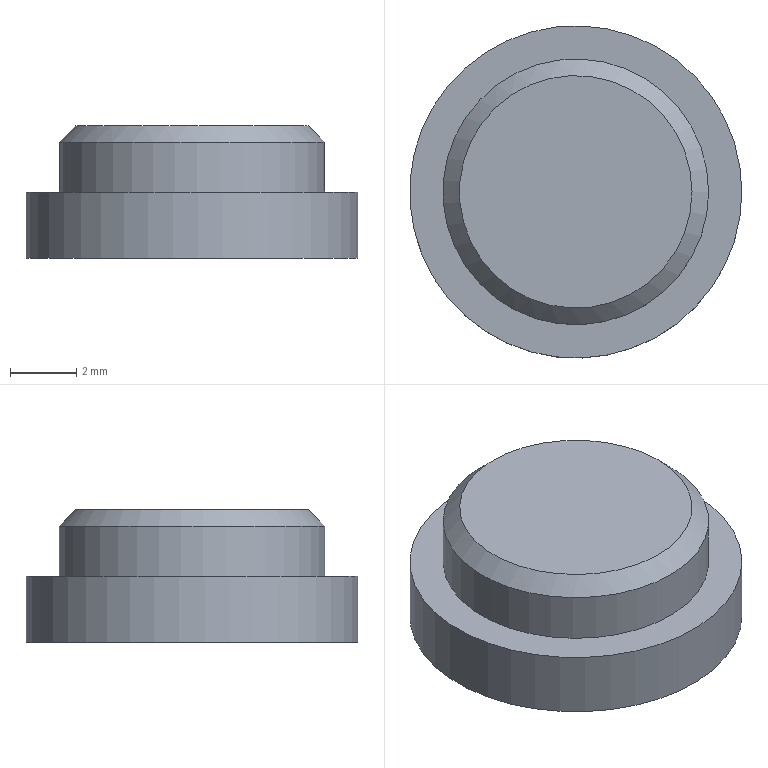Part | NX | features DATUM_CSYS 3, EXTRUDE 2, SKETCH 2, CHAMFER 1 | 2 solids | 8 faces | box 10 x 10 x 4 mm | volume 215.33 mm3 | plane 4 | cylinder 3 | cone 1 | commonest cylinder face diameters 5 x1 8 x1 10 x1
STEP:
#1=CARTESIAN_POINT('',(5.,0.,-2.));
#2=VERTEX_POINT('',#1);
#3=CARTESIAN_POINT('',(0.,0.,-2.));
#4=DIRECTION('',(0.,0.,-1.));
#5=DIRECTION('',(1.,0.,0.));
#6=AXIS2_PLACEMENT_3D('',#3,#4,#5);
#7=CIRCLE('',#6,5.);
#8=EDGE_CURVE('',#2,#2,#7,.T.);
#9=ORIENTED_EDGE('',*,*,#8,.F.);
#10=EDGE_LOOP('',(#9));
#11=FACE_BOUND('',#10,.T.);
#12=CARTESIAN_POINT('',(5.,0.,0.));
#13=VERTEX_POINT('',#12);
#14=CARTESIAN_POINT('',(0.,0.,0.));
#15=DIRECTION('',(0.,0.,-1.));
#16=DIRECTION('',(1.,0.,0.));
#17=AXIS2_PLACEMENT_3D('',#14,#15,#16);
#18=CIRCLE('',#17,5.);
#19=EDGE_CURVE('',#13,#13,#18,.T.);
#20=ORIENTED_EDGE('',*,*,#19,.T.);
#21=EDGE_LOOP('',(#20));
#22=FACE_BOUND('',#21,.T.);
#23=CARTESIAN_POINT('',(0.,0.,-2.));
#24=DIRECTION('',(0.,0.,1.));
#25=DIRECTION('',(1.,0.,0.));
#26=AXIS2_PLACEMENT_3D('',#23,#24,#25);
#27=CYLINDRICAL_SURFACE('',#26,5.);
#28=ADVANCED_FACE('',(#11,#22),#27,.T.);
#29=CARTESIAN_POINT('',(2.5,0.,-2.));
#30=VERTEX_POINT('',#29);
#31=CARTESIAN_POINT('',(0.,0.,-2.));
#32=DIRECTION('',(0.,0.,-1.));
#33=DIRECTION('',(1.,0.,0.));
#34=AXIS2_PLACEMENT_3D('',#31,#32,#33);
#35=CIRCLE('',#34,2.5);
#36=EDGE_CURVE('',#30,#30,#35,.T.);
#37=ORIENTED_EDGE('',*,*,#36,.T.);
#38=EDGE_LOOP('',(#37));
#39=FACE_BOUND('',#38,.T.);
#40=CARTESIAN_POINT('',(2.5,0.,0.));
#41=VERTEX_POINT('',#40);
#42=CARTESIAN_POINT('',(0.,0.,0.));
#43=DIRECTION('',(0.,0.,-1.));
#44=DIRECTION('',(1.,0.,0.));
#45=AXIS2_PLACEMENT_3D('',#42,#43,#44);
#46=CIRCLE('',#45,2.5);
#47=EDGE_CURVE('',#41,#41,#46,.T.);
#48=ORIENTED_EDGE('',*,*,#47,.F.);
#49=EDGE_LOOP('',(#48));
#50=FACE_BOUND('',#49,.T.);
#51=CARTESIAN_POINT('',(0.,0.,-2.));
#52=DIRECTION('',(0.,0.,1.));
#53=DIRECTION('',(1.,0.,0.));
#54=AXIS2_PLACEMENT_3D('',#51,#52,#53);
#55=CYLINDRICAL_SURFACE('',#54,2.5);
#56=ADVANCED_FACE('',(#39,#50),#55,.F.);
#57=ORIENTED_EDGE('',*,*,#8,.T.);
#58=EDGE_LOOP('',(#57));
#59=FACE_BOUND('',#58,.T.);
#60=ORIENTED_EDGE('',*,*,#36,.F.);
#61=EDGE_LOOP('',(#60));
#62=FACE_BOUND('',#61,.T.);
#63=CARTESIAN_POINT('',(0.,0.,-2.));
#64=DIRECTION('',(0.,0.,-1.));
#65=DIRECTION('',(-1.,0.,0.));
#66=AXIS2_PLACEMENT_3D('',#63,#64,#65);
#67=PLANE('',#66);
#68=ADVANCED_FACE('',(#59,#62),#67,.T.);
#69=ORIENTED_EDGE('',*,*,#19,.F.);
#70=EDGE_LOOP('',(#69));
#71=FACE_BOUND('',#70,.T.);
#72=ORIENTED_EDGE('',*,*,#47,.T.);
#73=EDGE_LOOP('',(#72));
#74=FACE_BOUND('',#73,.T.);
#75=CARTESIAN_POINT('',(0.,0.,0.));
#76=DIRECTION('',(0.,0.,-1.));
#77=DIRECTION('',(-1.,0.,0.));
#78=AXIS2_PLACEMENT_3D('',#75,#76,#77);
#79=PLANE('',#78);
#80=ADVANCED_FACE('',(#71,#74),#79,.F.);
#81=CLOSED_SHELL('',(#28,#56,#68,#80));
#82=MANIFOLD_SOLID_BREP('',#81);
#83=CARTESIAN_POINT('',(4.,0.,1.5));
#84=VERTEX_POINT('',#83);
#85=CARTESIAN_POINT('',(0.,0.,1.5));
#86=DIRECTION('',(0.,0.,1.));
#87=DIRECTION('',(1.,0.,0.));
#88=AXIS2_PLACEMENT_3D('',#85,#86,#87);
#89=CIRCLE('',#88,4.);
#90=EDGE_CURVE('',#84,#84,#89,.F.);
#91=ORIENTED_EDGE('',*,*,#90,.T.);
#92=EDGE_LOOP('',(#91));
#93=FACE_BOUND('',#92,.T.);
#94=CARTESIAN_POINT('',(4.,0.,0.));
#95=VERTEX_POINT('',#94);
#96=CARTESIAN_POINT('',(0.,0.,0.));
#97=DIRECTION('',(0.,0.,1.));
#98=DIRECTION('',(1.,0.,0.));
#99=AXIS2_PLACEMENT_3D('',#96,#97,#98);
#100=CIRCLE('',#99,4.);
#101=EDGE_CURVE('',#95,#95,#100,.T.);
#102=ORIENTED_EDGE('',*,*,#101,.T.);
#103=EDGE_LOOP('',(#102));
#104=FACE_BOUND('',#103,.T.);
#105=CARTESIAN_POINT('',(0.,0.,2.));
#106=DIRECTION('',(0.,0.,-1.));
#107=DIRECTION('',(-1.,0.,0.));
#108=AXIS2_PLACEMENT_3D('',#105,#106,#107);
#109=CYLINDRICAL_SURFACE('',#108,4.);
#110=ADVANCED_FACE('',(#93,#104),#109,.T.);
#111=CARTESIAN_POINT('',(3.5,0.,2.));
#112=VERTEX_POINT('',#111);
#113=CARTESIAN_POINT('',(0.,0.,2.));
#114=DIRECTION('',(0.,0.,1.));
#115=DIRECTION('',(1.,0.,0.));
#116=AXIS2_PLACEMENT_3D('',#113,#114,#115);
#117=CIRCLE('',#116,3.5);
#118=EDGE_CURVE('',#112,#112,#117,.T.);
#119=ORIENTED_EDGE('',*,*,#118,.T.);
#120=EDGE_LOOP('',(#119));
#121=FACE_BOUND('',#120,.T.);
#122=CARTESIAN_POINT('',(0.,0.,2.));
#123=DIRECTION('',(0.,0.,1.));
#124=DIRECTION('',(1.,0.,0.));
#125=AXIS2_PLACEMENT_3D('',#122,#123,#124);
#126=PLANE('',#125);
#127=ADVANCED_FACE('',(#121),#126,.T.);
#128=ORIENTED_EDGE('',*,*,#101,.F.);
#129=EDGE_LOOP('',(#128));
#130=FACE_BOUND('',#129,.T.);
#131=CARTESIAN_POINT('',(0.,0.,0.));
#132=DIRECTION('',(0.,0.,1.));
#133=DIRECTION('',(1.,0.,0.));
#134=AXIS2_PLACEMENT_3D('',#131,#132,#133);
#135=PLANE('',#134);
#136=ADVANCED_FACE('',(#130),#135,.F.);
#137=ORIENTED_EDGE('',*,*,#90,.F.);
#138=EDGE_LOOP('',(#137));
#139=FACE_BOUND('',#138,.T.);
#140=ORIENTED_EDGE('',*,*,#118,.F.);
#141=EDGE_LOOP('',(#140));
#142=FACE_BOUND('',#141,.T.);
#143=CARTESIAN_POINT('',(0.,0.,2.));
#144=DIRECTION('',(0.,0.,-1.));
#145=DIRECTION('',(-1.,0.,0.));
#146=AXIS2_PLACEMENT_3D('',#143,#144,#145);
#147=CONICAL_SURFACE('',#146,3.5,0.7854);
#148=ADVANCED_FACE('',(#139,#142),#147,.T.);
#149=CLOSED_SHELL('',(#110,#127,#136,#148));
#150=MANIFOLD_SOLID_BREP('',#149);
#151=(LENGTH_UNIT()NAMED_UNIT(*)SI_UNIT(.MILLI.,.METRE.));
#152=UNCERTAINTY_MEASURE_WITH_UNIT(LENGTH_MEASURE(0.00001),#151,'','');
#153=(NAMED_UNIT(*)PLANE_ANGLE_UNIT()SI_UNIT($,.RADIAN.));
#154=(NAMED_UNIT(*)SI_UNIT($,.STERADIAN.)SOLID_ANGLE_UNIT());
#155=(GEOMETRIC_REPRESENTATION_CONTEXT(3)GLOBAL_UNCERTAINTY_ASSIGNED_CONTEXT((#152))GLOBAL_UNIT_ASSIGNED_CONTEXT((#151,#153,#154))REPRESENTATION_CONTEXT('',''));
#156=ADVANCED_BREP_SHAPE_REPRESENTATION('',(#82,#150),#155);